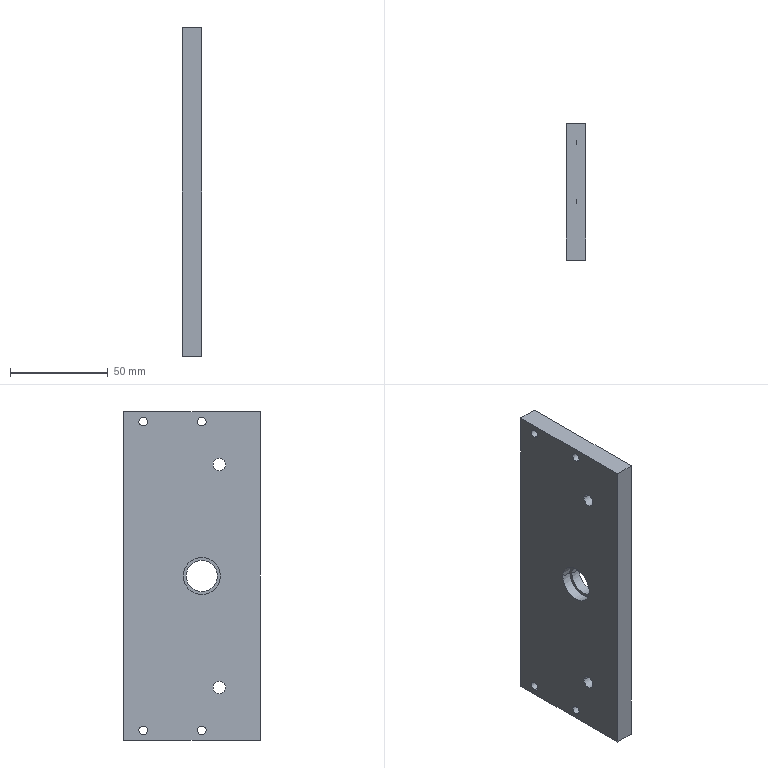Part | STEP file | 03-21 Lead screw fixing plate | 1 solid | 47 faces | box 10 x 70 x 168 mm | volume 112553 mm3 | cylinder 30 | plane 11 | cone 6 | commonest cylinder face diameters 4.5 x8 9 x8 3.3 x6 6.5 x4 16 x2 19 x2